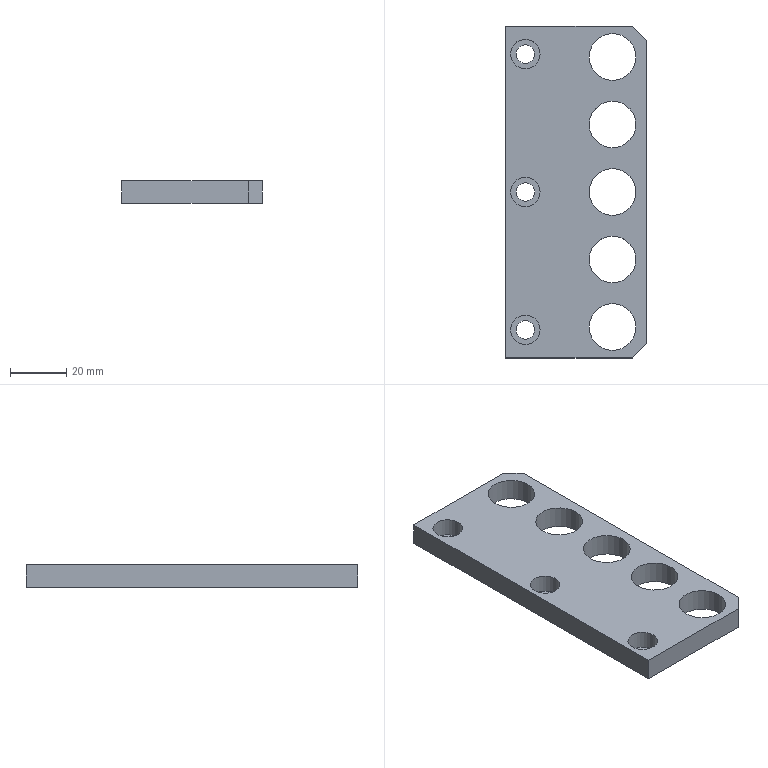NC program | NX | posted with a generic post | part box 50 x 118 x 8 mm
Lines 55 to 856 of 2555:
(ADAPTIVE_MILLING , TOOL : D8开粗)
N96 T04 M6
N98 G54
N100 G17 G0 G90 X50.236 Y10.179 S3500 M3
N102 G43 Z30. H4
N104 Z3.
N106 G94 G3 X50.236 Y10.179 Z2.605 I-2.237 J2.82 F1500.
N108 X50.236 Y10.179 Z2.21 I-2.237 J2.82
N110 X50.236 Y10.179 Z1.816 I-2.237 J2.82
N112 X50.236 Y10.179 Z1.421 I-2.237 J2.82
N114 X50.236 Y10.179 Z1.026 I-2.237 J2.82
N116 X50.236 Y10.179 Z0.631 I-2.237 J2.82
N118 X50.236 Y10.179 Z0.236 I-2.237 J2.82
N120 X50.236 Y10.179 Z-0.159 I-2.237 J2.82
N122 X50.236 Y10.179 Z-0.553 I-2.237 J2.82
N124 X50.236 Y10.179 Z-0.948 I-2.237 J2.82
N126 X50.236 Y10.179 Z-1.343 I-2.237 J2.82
N128 X50.236 Y10.179 Z-1.738 I-2.237 J2.82
N130 X50.236 Y10.179 Z-2.133 I-2.237 J2.82
N132 X50.236 Y10.179 Z-2.528 I-2.237 J2.82
N134 X50.236 Y10.179 Z-2.922 I-2.237 J2.82
N136 X50.236 Y10.179 Z-3.317 I-2.237 J2.82
N138 X50.236 Y10.179 Z-3.712 I-2.237 J2.82
N140 X50.236 Y10.179 Z-4.107 I-2.237 J2.82
N142 X50.236 Y10.179 Z-4.502 I-2.237 J2.82
N144 X50.236 Y10.179 Z-4.896 I-2.237 J2.82
N146 X50.236 Y10.179 Z-5.291 I-2.237 J2.82
N148 X50.236 Y10.179 Z-5.686 I-2.237 J2.82
N150 X50.236 Y10.179 Z-6.081 I-2.237 J2.82
N152 X50.236 Y10.179 Z-6.476 I-2.237 J2.82
N154 X50.236 Y10.179 Z-6.871 I-2.237 J2.82
N156 X50.236 Y10.179 Z-7.265 I-2.237 J2.82
N158 X50.236 Y10.179 Z-7.66 I-2.237 J2.82
N160 X50.236 Y10.179 Z-8.055 I-2.237 J2.82
N162 X50.236 Y10.179 Z-8.45 I-2.237 J2.82
N164 X50.236 Y10.179 Z-8.845 I-2.237 J2.82
N166 X47.998 Y16.599 Z-9. R3.6
N168 X51.279 Y11.397 R-3.625
N170 X44.716 Y11.182 R-3.701
N172 X49.182 Y16.615 R-3.777
N174 X45.263 Y10.239 R3.838
N176 X49.031 Y16.803 R-3.912
N178 X45.517 Y9.836 R3.976
N180 X49.277 Y16.867 R-4.046
N182 X45.642 Y9.575 R4.112
N184 X49.892 Y9.281 R4.161
N186 X44.448 Y15.226 R-4.182
N188 X44.68 Y10.442 R4.226
N190 X48.76 Y8.878 R4.238
N192 X51.89 Y11.457 R4.207
N194 X49.71 Y16.818 R4.18
N196 G1 X49.479 Y16.921
N198 G3 X48.429 Y16.246 R0.808
N200 G1 X48.303 Y15.168
N202 X48.286 Y15.019 Z-8.996
N204 X48.268 Y14.87 Z-8.985
N206 X48.251 Y14.721 Z-8.966
N208 X48.234 Y14.572 Z-8.939
N210 X48.216 Y14.423 Z-8.905
N212 X48.199 Y14.274 Z-8.862
N214 X48.181 Y14.125 Z-8.81
N216 X48.164 Y13.976 Z-8.75
N218 X48.147 Y13.827 Z-8.679
N220 X48.129 Y13.678 Z-8.598
N222 X48.112 Y13.529 Z-8.505
N224 X48.094 Y13.38 Z-8.4
N226 X48.077 Y13.231 Z-8.28
N228 X48.059 Y13.082 Z-8.142
N230 X48.042 Y12.933 Z-7.984
N232 X48.025 Y12.784 Z-7.8
N234 X48.007 Y12.635 Z-7.58
N236 X47.99 Y12.486 Z-7.308
N238 X47.972 Y12.337 Z-6.937
N240 X47.955 Y12.188 Z-6.
N242 G0 Z30.
N244 X26.236 Y10.182
N246 Z3.
N248 G3 X26.236 Y10.182 Z2.605 I-2.237 J2.82
N250 X26.236 Y10.182 Z2.21 I-2.237 J2.82
N252 X26.236 Y10.182 Z1.816 I-2.237 J2.82
N254 X26.236 Y10.182 Z1.421 I-2.237 J2.82
N256 X26.236 Y10.182 Z1.026 I-2.237 J2.82
N258 X26.236 Y10.182 Z0.631 I-2.237 J2.82
N260 X26.236 Y10.182 Z0.236 I-2.237 J2.82
N262 X26.236 Y10.182 Z-0.159 I-2.237 J2.82
N264 X26.236 Y10.182 Z-0.553 I-2.237 J2.82
N266 X26.236 Y10.182 Z-0.948 I-2.237 J2.82
N268 X26.236 Y10.182 Z-1.343 I-2.237 J2.82
N270 X26.236 Y10.182 Z-1.738 I-2.237 J2.82
N272 X26.236 Y10.182 Z-2.133 I-2.237 J2.82
N274 X26.236 Y10.182 Z-2.528 I-2.237 J2.82
N276 X26.236 Y10.182 Z-2.922 I-2.237 J2.82
N278 X26.236 Y10.182 Z-3.317 I-2.237 J2.82
N280 X26.236 Y10.182 Z-3.712 I-2.237 J2.82
N282 X26.236 Y10.182 Z-4.107 I-2.237 J2.82
N284 X26.236 Y10.182 Z-4.502 I-2.237 J2.82
N286 X26.236 Y10.182 Z-4.896 I-2.237 J2.82
N288 X26.236 Y10.182 Z-5.291 I-2.237 J2.82
N290 X26.236 Y10.182 Z-5.686 I-2.237 J2.82
N292 X26.236 Y10.182 Z-6.081 I-2.237 J2.82
N294 X26.236 Y10.182 Z-6.476 I-2.237 J2.82
N296 X26.236 Y10.182 Z-6.871 I-2.237 J2.82
N298 X26.236 Y10.182 Z-7.265 I-2.237 J2.82
N300 X26.236 Y10.182 Z-7.66 I-2.237 J2.82
N302 X26.236 Y10.182 Z-8.055 I-2.237 J2.82
N304 X26.236 Y10.182 Z-8.45 I-2.237 J2.82
N306 X26.236 Y10.182 Z-8.845 I-2.237 J2.82
N308 X23.999 Y16.602 Z-9. R3.6
N310 X27.28 Y11.4 R-3.625
N312 X20.716 Y11.186 R-3.701
N314 X25.184 Y16.62 R-3.778
N316 X21.42 Y10.095 R3.84
N318 X25.242 Y16.743 R-3.913
N320 X21.691 Y9.71 R3.978
N322 X25.282 Y16.871 R-4.048
N324 X21.826 Y9.459 R4.114
N326 X25.888 Y9.282 R4.161
N328 X21.511 Y16.374 R-4.181
N330 X27.568 Y15.195 R-4.189
N332 X26.569 Y16.317 R4.309
N334 X25.324 Y15.974 R0.808
N336 G1 X24.935 Y14.99
N338 X24.879 Y14.851 Z-8.996
N340 X24.824 Y14.711 Z-8.985
N342 X24.769 Y14.572 Z-8.966
N344 X24.714 Y14.432 Z-8.939
N346 X24.659 Y14.293 Z-8.905
N348 X24.604 Y14.153 Z-8.862
N350 X24.548 Y14.014 Z-8.81
N352 X24.493 Y13.874 Z-8.75
N354 X24.438 Y13.735 Z-8.679
N356 X24.383 Y13.595 Z-8.598
N358 X24.328 Y13.456 Z-8.505
N360 X24.273 Y13.316 Z-8.4
N362 X24.217 Y13.177 Z-8.28
N364 X24.162 Y13.037 Z-8.142
N366 X24.107 Y12.898 Z-7.984
N368 X24.052 Y12.758 Z-7.8
N370 X23.997 Y12.619 Z-7.58
N372 X23.942 Y12.479 Z-7.308
N374 X23.887 Y12.34 Z-6.937
N376 X23.831 Y12.2 Z-6.
N378 G0 Z30.
N380 X2.234 Y10.181
N382 Z3.
N384 G3 X2.234 Y10.181 Z2.605 I-2.237 J2.82
N386 X2.234 Y10.181 Z2.21 I-2.237 J2.82
N388 X2.234 Y10.181 Z1.816 I-2.237 J2.82
N390 X2.234 Y10.181 Z1.421 I-2.237 J2.82
N392 X2.234 Y10.181 Z1.026 I-2.237 J2.82
N394 X2.234 Y10.181 Z0.631 I-2.237 J2.82
N396 X2.234 Y10.181 Z0.236 I-2.237 J2.82
N398 X2.234 Y10.181 Z-0.159 I-2.237 J2.82
N400 X2.234 Y10.181 Z-0.553 I-2.237 J2.82
N402 X2.234 Y10.181 Z-0.948 I-2.237 J2.82
N404 X2.234 Y10.181 Z-1.343 I-2.237 J2.82
N406 X2.234 Y10.181 Z-1.738 I-2.237 J2.82
N408 X2.234 Y10.181 Z-2.133 I-2.237 J2.82
N410 X2.234 Y10.181 Z-2.528 I-2.237 J2.82
N412 X2.234 Y10.181 Z-2.922 I-2.237 J2.82
N414 X2.234 Y10.181 Z-3.317 I-2.237 J2.82
N416 X2.234 Y10.181 Z-3.712 I-2.237 J2.82
N418 X2.234 Y10.181 Z-4.107 I-2.237 J2.82
N420 X2.234 Y10.181 Z-4.502 I-2.237 J2.82
N422 X2.234 Y10.181 Z-4.896 I-2.237 J2.82
N424 X2.234 Y10.181 Z-5.291 I-2.237 J2.82
N426 X2.234 Y10.181 Z-5.686 I-2.237 J2.82
N428 X2.234 Y10.181 Z-6.081 I-2.237 J2.82
N430 X2.234 Y10.181 Z-6.476 I-2.237 J2.82
N432 X2.234 Y10.181 Z-6.871 I-2.237 J2.82
N434 X2.234 Y10.181 Z-7.265 I-2.237 J2.82
N436 X2.234 Y10.181 Z-7.66 I-2.237 J2.82
N438 X2.234 Y10.181 Z-8.055 I-2.237 J2.82
N440 X2.234 Y10.181 Z-8.45 I-2.237 J2.82
N442 X2.234 Y10.181 Z-8.845 I-2.237 J2.82
N444 X-0.003 Y16.601 Z-9. R3.6
N446 X3.277 Y11.399 R-3.625
N448 X-3.285 Y11.184 R-3.701
N450 X1.18 Y16.617 R-3.777
N452 X-2.739 Y10.241 R3.838
N454 X1.029 Y16.805 R-3.912
N456 X-2.125 Y9.586 R3.977
N458 X1.064 Y16.936 R-4.048
N460 X-2.172 Y9.455 R4.114
N462 X1.269 Y9.031 R4.161
N464 X-3.945 Y14.399 R-4.177
N466 X3.077 Y15.84 R-4.187
N468 X1.752 Y16.81 R4.235
N470 X0.622 Y16.2 R0.808
N472 G1 X0.455 Y15.146
N474 X0.432 Y14.998 Z-8.996
N476 X0.408 Y14.85 Z-8.985
N478 X0.385 Y14.702 Z-8.966
N480 X0.361 Y14.554 Z-8.939
N482 X0.338 Y14.406 Z-8.905
N484 X0.314 Y14.257 Z-8.862
N486 X0.291 Y14.109 Z-8.81
N488 X0.268 Y13.961 Z-8.75
N490 X0.244 Y13.813 Z-8.679
N492 X0.221 Y13.665 Z-8.598
N494 X0.197 Y13.517 Z-8.505
N496 X0.174 Y13.369 Z-8.4
N498 X0.15 Y13.22 Z-8.28
N500 X0.127 Y13.072 Z-8.142
N502 X0.104 Y12.924 Z-7.984
N504 X0.08 Y12.776 Z-7.8
N506 X0.057 Y12.628 Z-7.58
N508 X0.033 Y12.48 Z-7.308
N510 X0.01 Y12.331 Z-6.937
N512 X-0.013 Y12.183 Z-6.
N514 G0 Z30.
N516 X0.506 Y-39.041
N518 Z-6.
N520 G1 X0.507 Y-38.891 Z-6.937
N522 X0.509 Y-38.741 Z-7.308
N524 X0.51 Y-38.591 Z-7.58
N526 X0.512 Y-38.441 Z-7.8
N528 X0.513 Y-38.291 Z-7.984
N530 X0.514 Y-38.141 Z-8.142
N532 X0.516 Y-37.991 Z-8.28
N534 X0.517 Y-37.841 Z-8.4
N536 X0.519 Y-37.691 Z-8.505
N538 X0.52 Y-37.541 Z-8.598
N540 X0.522 Y-37.391 Z-8.679
N542 X0.523 Y-37.241 Z-8.75
N544 X0.525 Y-37.091 Z-8.81
N546 X0.526 Y-36.941 Z-8.862
N548 X0.528 Y-36.791 Z-8.905
N550 X0.529 Y-36.641 Z-8.939
N552 X0.53 Y-36.491 Z-8.966
N554 X0.532 Y-36.341 Z-8.985
N556 X0.533 Y-36.191 Z-8.996
N558 X0.535 Y-36.041 Z-9.
N560 X0.547 Y-34.792
N562 G3 X-0.008 Y-34.016 R0.808
N564 X-2.484 Y-33.75 R10.653
N566 X-8.994 Y-33.699 R394.13
N568 G1 X-61.118 Y-33.698
N570 G2 X-64.699 Y-31.591 R4.579
N572 X-65.979 Y-27.829 R8.408
N574 X-66.193 Y-22.211 R50.658
N576 G1 X-66.198 Y-18.011
N578 X-66.197 Y28.592
N580 G2 X-64.179 Y32.122 R4.565
N582 X-60.411 Y33.465 R8.23
N584 X-55.394 Y33.69 R42.849
N586 G1 X-50.444 Y33.699
N588 X61.106 Y33.698
N590 G2 X64.711 Y31.557 R4.596
N592 X65.982 Y27.78 R8.5
N594 X66.193 Y22.2 R50.827
N596 G1 X66.198 Y18.
N598 X66.197 Y-28.603
N600 G2 X64.092 Y-32.187 R4.584
N602 X60.338 Y-33.476 R8.406
N604 X54.72 Y-33.694 R49.804
N606 G1 X50.52 Y-33.699
N608 X1.745 Y-33.698
N610 G3 X-2.839 Y-33.457 R703.994
N612 X-10.268 Y-33.4 R435.247
N614 G1 X-59.656 Y-33.398
N616 G2 X-64.449 Y-30.442 R5.687
N618 X-65.692 Y-26.187 R10.577
N620 X-65.894 Y-20.043 R64.975
N622 G1 X-65.898 Y-16.743
N624 X-65.896 Y27.129
N626 G2 X-62.928 Y31.949 R5.7
N628 X-58.858 Y33.171 R10.376
N630 X-53.24 Y33.391 R54.557
N632 G1 X-49.115 Y33.399
N634 X59.64 Y33.397
N636 G2 X64.451 Y30.427 R5.7
N638 X65.674 Y26.324 R10.42
N640 X65.891 Y20.668 R55.859
N642 G1 X65.898 Y16.131
N644 X65.896 Y-27.14
N646 G2 X62.977 Y-31.922 R5.688
N648 X58.88 Y-33.169 R10.292
N650 X53.3 Y-33.391 R53.72
N652 G1 X49.175 Y-33.399
N654 X2.745 Y-33.396
N656 G2 X-3.054 Y-33.162 R769.478
N658 G3 X-11.206 Y-33.1 R473.739
N660 G1 X-58.381 Y-33.097
N662 G2 X-64.217 Y-29.458 R6.453
N664 X-65.394 Y-24.989 R12.24
N666 X-65.595 Y-18.094 R78.796
N668 G1 X-65.598 Y-14.382
N670 X-65.596 Y25.854
N672 G2 X-61.883 Y31.75 R6.483
N674 X-57.515 Y32.89 R12.302
N676 X-51.071 Y33.094 R72.384
N678 G1 X-47.771 Y33.098
N680 X58.365 Y33.097
N682 G2 X64.241 Y29.4 R6.471
N684 X65.387 Y25.036 R12.262
N686 X65.594 Y18.179 R76.142
N688 G1 X65.598 Y14.466
N690 X65.596 Y-25.865
N692 G2 X61.894 Y-31.747 R6.473
N694 X57.417 Y-32.9 R12.435
N696 X51.16 Y-33.094 R73.915
N698 G1 X47.86 Y-33.098
N700 X3.645 Y-33.096
N702 G2 X-3.124 Y-32.868 R440.519
N704 G3 X-11.918 Y-32.8 R494.43
N706 G1 X-57.168 Y-32.798
N708 G2 X-61.748 Y-31.398 R7.3
N710 X-64.538 Y-27.089 R8.183
N712 X-65.216 Y-22.123 R20.919
N714 X-65.298 Y-13.048 R277.677
N716 G1 X-65.296 Y24.692
N718 G2 X-63.836 Y29.32 R7.265
N720 X-59.558 Y32.045 R8.231
N722 X-54.516 Y32.72 R21.269
N724 X-45.929 Y32.798 R280.799
N726 G1 X57.146 Y32.797
N728 G2 X61.604 Y31.5 R7.358
N730 X64.495 Y27.22 R8.063
N732 X65.205 Y22.335 R19.927
N734 X65.298 Y13.373 R240.548
N736 G1 X65.296 Y-24.703
N738 G2 X63.784 Y-29.388 R7.242
N740 X59.421 Y-32.084 R8.332
N742 X54.56 Y-32.718 R21.674
N744 X45.823 Y-32.798 R276.552
N746 G1 X4.883
N748 G2 X-3.231 Y-32.571 R325.759
N750 G3 X-11.806 Y-32.5 R535.192
N752 G1 X-55.944 Y-32.499
N754 G2 X-59.694 Y-31.897 R9.494
N756 X-63.796 Y-27.611 R7.681
N758 X-64.814 Y-22.863 R15.69
N760 X-64.995 Y-15.329 R103.821
N762 G1 X-64.997 Y-12.029
N764 X-64.996 Y23.642
N766 G2 X-64.186 Y27.647 R8.751
N768 X-59.895 Y31.381 R7.847
N770 X-55.019 Y32.34 R16.701
N772 X-47.672 Y32.496 R117.542
N774 G1 X-44.785 Y32.498
N776 X56.152 Y32.496
N778 G2 X60.189 Y31.665 R8.695
N780 X63.885 Y27.383 R7.856
N782 X64.834 Y22.581 R16.635
N784 X64.995 Y15.197 R114.549
N786 G1 X64.997 Y11.897
N788 X64.996 Y-23.578
N790 G2 X64.279 Y-27.454 R8.997
N792 X59.975 Y-31.35 R7.776
N794 X55.178 Y-32.328 R16.273
N796 X47.119 Y-32.497 R119.876
N798 G1 X5.783 Y-32.498
N800 G2 X-3.449 Y-32.271 R353.509
N802 G3 X-12.818 Y-32.2 R603.998
N804 G1 X-55.106 Y-32.199
N806 G2 X-58.942 Y-31.636 R10.675
N808 X-63.378 Y-27.239 R7.929
N810 X-64.482 Y-22.397 R15.638
N812 X-64.694 Y-14.527 R97.762
N814 G1 X-64.697 Y-10.477
N816 X-64.696 Y22.554
N818 G2 X-64.15 Y26.394 R10.845
N820 X-59.743 Y30.874 R7.92
N822 X-54.715 Y31.999 R15.91
N824 X-47.482 Y32.194 R96.259
N826 G1 X-44.182 Y32.198
N828 X55.139 Y32.196
N830 G2 X58.974 Y31.62 R10.548
N832 X63.39 Y27.203 R7.945
N834 X64.501 Y22.17 R16.064
N836 X64.693 Y14.787 R100.086
N838 G1 X64.697 Y10.662
N840 X64.695 Y-22.64
N842 G2 X64.093 Y-26.544 R10.467
N844 X59.721 Y-30.884 R7.949
N846 X54.911 Y-31.981 R15.644
N848 X47.566 Y-32.194 R90.033
N850 G1 X44.266 Y-32.198
N852 X5.82 Y-32.196
N854 G2 X-4.038 Y-31.962 R549.5
N856 G3 X-12.968 Y-31.9 R639.08
N858 G1 X-54.056 Y-31.899
N860 G2 X-57.917 Y-31.47 R13.202
N862 X-62.997 Y-26.818 R8.147
N864 X-64.16 Y-21.875 R15.842
N866 X-64.389 Y-14.831 R83.45
N868 G1 X-64.397 Y-9.506
N870 X-64.395 Y21.719
N872 G2 X-63.906 Y25.609 R12.287
N874 X-59.313 Y30.497 R8.165
N876 X-54.295 Y31.668 R15.966
N878 X-46.764 Y31.893 R90.426
N880 G1 X-43.464 Y31.897
N882 X54.315 Y31.895
N884 G2 X58.234 Y31.364 R11.835
N886 X63.01 Y26.782 R8.183
N888 X64.163 Y21.837 R15.972
N890 X64.389 Y14.718 R84.962
N892 G1 X64.397 Y9.318
N894 X64.388 Y-22.653
N896 G2 X63.195 Y-27.17 R9.198
N898 X58.589 Y-30.789 R8.684
N900 X53.443 Y-31.737 R18.895
N902 X45.346 Y-31.896 R135.04
N904 G1 X7.433 Y-31.898
N906 G2 X-3.371 Y-31.679 R375.458
N908 G3 X-12.744 Y-31.601 R637.098
N910 G1 X-53.231 Y-31.599
N912 G2 X-57.175 Y-31.209 R14.957
N914 X-61.632 Y-28.13 R8.098
N916 G1 X-62.206 Y-27.556
N918 X-62.694 Y-26.779
N920 G2 X-63.913 Y-20.641 R21.436
N922 X-64.092 Y-12.844 R123.731
N924 G1 X-64.097 Y-8.794
N926 X-64.095 Y20.867
N928 G2 X-63.658 Y24.841 R14.049
N930 X-58.868 Y30.14 R8.396
N932 X-53.819 Y31.346 R16.185
N934 X-45.988 Y31.592 R88.752
N936 G1 X-41.863 Y31.597
N938 X53.452 Y31.595
N940 G2 X57.423 Y31.134 R13.608
N942 X62.656 Y26.33 R8.411
N944 X63.848 Y21.278 R16.311
N946 X64.088 Y13.934 R85.558
N948 G1 X64.096 Y8.61
N950 X64.095 Y-22.453
N952 G2 X62.534 Y-27.202 R9.265
N954 X57.722 Y-30.583 R9.267
N956 X52.483 Y-31.451 R21.049
N958 X42.585 Y-31.597 R188.242
N960 G1 X6.898 Y-31.596
N962 G2 X-3.999 Y-31.369 R550.68
N964 G3 X-13.269 Y-31.301 R647.104
N966 G1 X-52.331 Y-31.3
N968 G2 X-56.285 Y-30.984 R17.939
N970 X-60.293 Y-28.883 R9.158
N972 X-61.556 Y-28.206 R4.98
N974 G1 X-62.206 Y-27.556
N976 X-62.694 Y-26.779
N978 X-62.997 Y-25.912
N980 G2 X-63.575 Y-20.794 R161.787
N982 X-63.792 Y-11.724 R131.889
N984 G1 X-63.796 Y-7.449
N986 X-63.795 Y19.967
N988 G2 X-63.421 Y24.026 R16.509
N990 X-58.473 Y29.772 R8.603
N992 X-53.395 Y31.021 R16.295
N994 X-46.091 Y31.288 R78.704
N996 G1 X-41.028 Y31.297
N998 X52.627 Y31.295
N1000 G2 X56.717 Y30.871 R15.336
N1002 X62.268 Y25.981 R8.606
N1004 X63.529 Y20.793 R16.411
N1006 X63.787 Y13.15 R85.647
N1008 G1 X63.796 Y8.2
N1010 X63.795 Y-22.45
N1012 G2 X63.072 Y-25.258 R13.964
N1014 G1 X63.002 Y-25.889
N1016 G2 X62.249 Y-27.501 R4.767
N1018 X60.884 Y-28.641 R4.767
N1020 X54.012 Y-30.958 R16.079
N1022 X47.011 Y-31.282 R64.531
N1024 G1 X40.973 Y-31.297
N1026 X7.461 Y-31.296
N1028 G2 X-4.48 Y-31.063 R634.025
N1030 G3 X-13.793 Y-31.001 R655.45
N1032 G1 X-51.506 Y-31.
N1034 G2 X-55.686 Y-30.689 R19.936
N1036 X-59.197 Y-29.18 R11.272
N1038 G3 X-59.912 Y-28.997 R1.401
N1040 G1 X-60.779 Y-28.694
N1042 X-61.556 Y-28.206
N1044 X-62.206 Y-27.556
N1046 X-62.694 Y-26.779
N1048 X-62.997 Y-25.912
N1050 G2 X-63.102 Y-23.654 R12.983
N1052 X-63.449 Y-16.244 R192.047
N1054 X-63.496 Y-6.644 R677.077
N1056 G1 X-63.495 Y19.131
N1058 G2 X-63.165 Y23.271 R18.98
N1060 X-58.014 Y29.443 R8.819
N1062 X-52.753 Y30.721 R16.806
N1064 X-45.148 Y30.989 R83.609
N1066 G1 X-40.198 Y30.997
N1068 X51.727 Y30.996
N1070 G2 X55.902 Y30.636 R18.017
N1072 X61.933 Y25.534 R8.815
N1074 X63.224 Y20.2 R16.866
N1076 X63.487 Y12.219 R90.237
N1078 G1 X63.496 Y6.819
N1080 X63.494 Y-22.443
N1082 X63.1 Y-24.093
N1084 G2 X63.071 Y-25.262 R9.795
N1086 G3 X63.58 Y-26.103 R0.808
N1088 G1 X64.859 Y-26.602
N1090 X64.998 Y-26.656 Z-8.996
N1092 X65.138 Y-26.711 Z-8.985
N1094 X65.278 Y-26.766 Z-8.966
N1096 X65.417 Y-26.82 Z-8.939
N1098 X65.557 Y-26.875 Z-8.905
N1100 X65.697 Y-26.929 Z-8.862
N1102 X65.837 Y-26.984 Z-8.81
N1104 X65.976 Y-27.038 Z-8.75
N1106 X66.116 Y-27.093 Z-8.679
N1108 X66.256 Y-27.148 Z-8.598
N1110 X66.395 Y-27.202 Z-8.505
N1112 X66.535 Y-27.257 Z-8.4
N1114 X66.675 Y-27.311 Z-8.28
N1116 X66.815 Y-27.366 Z-8.142
N1118 X66.954 Y-27.421 Z-7.984
N1120 X67.094 Y-27.475 Z-7.8
N1122 X67.234 Y-27.53 Z-7.58
N1124 X67.373 Y-27.584 Z-7.308
N1126 X67.513 Y-27.639 Z-6.937
N1128 X67.653 Y-27.693 Z-6.
N1130 G0 Z30.
N1132 X-67.881 Y-23.617
N1134 Z-6.
N1136 G1 X-67.741 Y-23.671 Z-6.937
N1138 X-67.602 Y-23.726 Z-7.308
N1140 X-67.462 Y-23.78 Z-7.58
N1142 X-67.322 Y-23.835 Z-7.8
N1144 X-67.183 Y-23.89 Z-7.984
N1146 X-67.043 Y-23.944 Z-8.142
N1148 X-66.903 Y-23.999 Z-8.28
N1150 X-66.763 Y-24.053 Z-8.4
N1152 X-66.624 Y-24.108 Z-8.505
N1154 X-66.484 Y-24.162 Z-8.598
N1156 X-66.344 Y-24.217 Z-8.679
N1158 X-66.204 Y-24.272 Z-8.75
N1160 X-66.065 Y-24.326 Z-8.81
N1162 X-65.925 Y-24.381 Z-8.862
N1164 X-65.785 Y-24.435 Z-8.905
N1166 X-65.646 Y-24.49 Z-8.939
N1168 X-65.506 Y-24.544 Z-8.966
N1170 X-65.366 Y-24.599 Z-8.985
N1172 X-65.226 Y-24.654 Z-8.996
N1174 X-65.087 Y-24.708 Z-9.
N1176 G3 X-64.62 Y-24.745 R0.821
N1178 G1 X-63.735 Y-24.551
N1180 G3 X-63.1 Y-23.762 R0.808
N1182 X-63.186 Y-12.277 R757.047
N1184 G1 X-63.196 Y-7.027
N1186 X-63.194 Y18.46
N1188 G2 X-62.858 Y22.751 R20.089
N1190 X-57.536 Y29.129 R9.028
N1192 X-52.087 Y30.427 R17.438
N1194 X-44.144 Y30.689 R90.646
N1196 G1 X-38.819 Y30.697
N1198 X50.977 Y30.695
N1200 G2 X55.194 Y30.371 R20.248
N1202 X61.633 Y25.025 R9.029
N1204 X62.605 Y21.917 R16.705
N1206 X63.021 Y20.798 R4.271
N1208 X63.1 Y18.349 R16.852
N1210 X63.196 Y5.708 R594.316
N1212 G1 X63.194 Y-21.755
N1214 X63.1 Y-22.369
N1216 Y-24.094
N1218 G3 X64.658 Y-24.35 R0.8
N1220 G1 X65.083 Y-22.818 Z-8.9
N1222 X65.201 Y-22.406 F15000.
N1224 X65.305 Y-21.989
N1226 X65.313 Y-21.882
N1228 Y16.137
N1230 X65.303 Y16.244
N1232 X65.284 Y16.35
N1234 X65.09 Y17.048
N1236 X64.666 Y18.58 Z-9. F1500.
N1238 G3 X63.1 Y18.349 R0.8
N1240 G1 Y-25.001
N1242 G2 X62.714 Y-26.736 R4.764
N1244 X61.629 Y-28.146 R4.767
N1246 X60.048 Y-28.964 R4.764
N1248 X51.534 Y-30.833 R25.207
N1250 X42.274 Y-30.996 R166.344
N1252 G1 X8.837 Y-30.997
N1254 G2 X-3.923 Y-30.775 R514.516
N1256 G3 X-14.656 Y-30.701 R680.231
N1258 G1 X-50.756 Y-30.7
N1260 G2 X-55.014 Y-30.412 R22.291
N1262 X-58.352 Y-29.226 R15.336
N1264 G3 X-59.001 Y-29.1 R1.258
N1266 X-59.753 Y-29.038 R13.408
N1268 G1 X-60.795 Y-29.171
N1270 G3 X-60.96 Y-30.736 R0.808
N1272 G1 X-60.818 Y-30.785 Z-8.996
N1274 X-60.677 Y-30.835 Z-8.985
N1276 X-60.535 Y-30.884 Z-8.966
N1278 X-60.393 Y-30.934 Z-8.939
N1280 X-60.252 Y-30.983 Z-8.905
N1282 X-60.11 Y-31.033 Z-8.862
N1284 X-59.969 Y-31.082 Z-8.81
N1286 X-59.827 Y-31.132 Z-8.75
N1288 X-59.686 Y-31.181 Z-8.679
N1290 X-59.544 Y-31.231 Z-8.598
N1292 X-59.402 Y-31.281 Z-8.505
N1294 X-59.261 Y-31.33 Z-8.4
N1296 X-59.119 Y-31.38 Z-8.28
N1298 X-58.978 Y-31.429 Z-8.142
N1300 X-58.836 Y-31.479 Z-7.984
N1302 X-58.694 Y-31.528 Z-7.8
N1304 X-58.553 Y-31.578 Z-7.58
N1306 X-58.411 Y-31.627 Z-7.308
N1308 X-58.27 Y-31.677 Z-6.937
N1310 X-58.128 Y-31.726 Z-6.
N1312 G0 Z30.
N1314 X58.764 Y-31.588
N1316 Z-6.
N1318 G1 X58.904 Y-31.534 Z-6.937
N1320 X59.044 Y-31.48 Z-7.308
N1322 X59.184 Y-31.426 Z-7.58
N1324 X59.324 Y-31.372 Z-7.8
N1326 X59.464 Y-31.318 Z-7.984
N1328 X59.604 Y-31.264 Z-8.142
N1330 X59.743 Y-31.21 Z-8.28
N1332 X59.883 Y-31.156 Z-8.4
N1334 X60.023 Y-31.102 Z-8.505
N1336 X60.163 Y-31.048 Z-8.598
N1338 X60.303 Y-30.995 Z-8.679
N1340 X60.443 Y-30.941 Z-8.75
N1342 X60.583 Y-30.887 Z-8.81
N1344 X60.723 Y-30.833 Z-8.862
N1346 X60.863 Y-30.779 Z-8.905
N1348 X61.003 Y-30.725 Z-8.939
N1350 X61.143 Y-30.671 Z-8.966
N1352 X61.283 Y-30.617 Z-8.985
N1354 X61.423 Y-30.563 Z-8.996
N1356 X61.563 Y-30.509 Z-9.
N1358 G3 X61.271 Y-28.947 R0.808
N1360 G1 X60.048 Y-28.964
N1362 G3 X56.651 Y-29.77 R69.655
N1364 G2 X48.987 Y-30.623 R38.617
N1366 X39.687 Y-30.696 R423.148
N1368 G1 X8.2 Y-30.695
N1370 G2 X-4.369 Y-30.47 R687.903
N1372 G3 X-16.006 Y-30.401 R715.492
N1374 G1 X-56.406
N1376 X-56.694 Y-30.348
N1378 X-58.89 Y-29.511
N1380 G3 X-59.269 Y-31.069 R-0.808
N1382 G1 X-59.12 Y-31.086 Z-8.996
N1384 X-58.97 Y-31.103 Z-8.985
N1386 X-58.821 Y-31.119 Z-8.966
N1388 X-58.672 Y-31.136 Z-8.939
N1390 X-58.523 Y-31.153 Z-8.905
N1392 X-58.374 Y-31.17 Z-8.862
N1394 X-58.225 Y-31.187 Z-8.81
N1396 X-58.076 Y-31.203 Z-8.75
N1398 X-57.927 Y-31.22 Z-8.679
N1400 X-57.778 Y-31.237 Z-8.598
N1402 X-57.629 Y-31.254 Z-8.505
N1404 X-57.48 Y-31.271 Z-8.4
N1406 X-57.331 Y-31.287 Z-8.28
N1408 X-57.182 Y-31.304 Z-8.142
N1410 X-57.033 Y-31.321 Z-7.984
N1412 X-56.884 Y-31.338 Z-7.8
N1414 X-56.735 Y-31.355 Z-7.58
N1416 X-56.586 Y-31.371 Z-7.308
N1418 X-56.437 Y-31.388 Z-6.937
N1420 X-56.287 Y-31.405 Z-6.
N1422 G0 Z30.
N1424 X58.119 Y-31.837
N1426 Z-6.
N1428 G1 X58.259 Y-31.783 Z-6.937
N1430 X58.399 Y-31.729 Z-7.308
N1432 X58.539 Y-31.675 Z-7.58
N1434 X58.678 Y-31.621 Z-7.8
N1436 X58.818 Y-31.567 Z-7.984
N1438 X58.958 Y-31.513 Z-8.142
N1440 X59.098 Y-31.459 Z-8.28
N1442 X59.238 Y-31.405 Z-8.4
N1444 X59.378 Y-31.351 Z-8.505
N1446 X59.518 Y-31.297 Z-8.598
N1448 X59.658 Y-31.243 Z-8.679
N1450 X59.798 Y-31.189 Z-8.75
N1452 X59.938 Y-31.135 Z-8.81
N1454 X60.078 Y-31.081 Z-8.862
N1456 X60.218 Y-31.027 Z-8.905
N1458 X60.358 Y-30.973 Z-8.939
N1460 X60.498 Y-30.919 Z-8.966
N1462 X60.638 Y-30.866 Z-8.985
N1464 X60.778 Y-30.812 Z-8.996
N1466 X60.918 Y-30.758 Z-9.
N1468 G3 X60.728 Y-29.202 R0.808
N1470 G1 X59.528 Y-29.066
N1472 G3 X56.363 Y-29.539 R21.375
N1474 G2 X47.336 Y-30.349 R51.747
N1476 X38.261 Y-30.396 R658.085
N1478 G1 X-54.484 Y-30.394
N1480 G2 X-56.42 Y-29.693 R14.547
N1482 G3 X-58. Y-29.104 R11.805
N1484 X-58.986 Y-29.123 R9.512
N1486 G1 X-60.107 Y-29.399
N1488 G3 X-60.004 Y-30.986 R0.808
N1490 G1 X-59.855 Y-31.003 Z-8.996
N1492 X-59.706 Y-31.02 Z-8.985
N1494 X-59.557 Y-31.037 Z-8.966
N1496 X-59.408 Y-31.053 Z-8.939
N1498 X-59.259 Y-31.07 Z-8.905
N1500 X-59.11 Y-31.087 Z-8.862
N1502 X-58.961 Y-31.104 Z-8.81
N1504 X-58.812 Y-31.121 Z-8.75
N1506 X-58.663 Y-31.137 Z-8.679
N1508 X-58.514 Y-31.154 Z-8.598
N1510 X-58.365 Y-31.171 Z-8.505
N1512 X-58.216 Y-31.188 Z-8.4
N1514 X-58.067 Y-31.204 Z-8.28
N1516 X-57.917 Y-31.221 Z-8.142
N1518 X-57.768 Y-31.238 Z-7.984
N1520 X-57.619 Y-31.255 Z-7.8
N1522 X-57.47 Y-31.272 Z-7.58
N1524 X-57.321 Y-31.288 Z-7.308
N1526 X-57.172 Y-31.305 Z-6.937
N1528 X-57.023 Y-31.322 Z-6.
N1530 G0 Z30.
N1532 X57.318 Y-31.525
N1534 Z-6.
N1536 G1 X57.465 Y-31.496 Z-6.937
N1538 X57.612 Y-31.467 Z-7.308
N1540 X57.759 Y-31.438 Z-7.58
N1542 X57.906 Y-31.409 Z-7.8
N1544 X58.054 Y-31.38 Z-7.984
N1546 X58.201 Y-31.351 Z-8.142
N1548 X58.348 Y-31.322 Z-8.28
N1550 X58.495 Y-31.293 Z-8.4
N1552 X58.642 Y-31.264 Z-8.505
N1554 X58.79 Y-31.235 Z-8.598
N1556 X58.937 Y-31.207 Z-8.679
N1558 X59.084 Y-31.178 Z-8.75
N1560 X59.231 Y-31.149 Z-8.81
N1562 X59.378 Y-31.12 Z-8.862
N1564 X59.525 Y-31.091 Z-8.905
N1566 X59.673 Y-31.062 Z-8.939
N1568 X59.82 Y-31.033 Z-8.966
N1570 X59.967 Y-31.004 Z-8.985
N1572 X60.114 Y-30.975 Z-8.996
N1574 X60.261 Y-30.946 Z-9.
N1576 G3 X60.281 Y-29.365 R0.808
N1578 G1 X59. Y-29.1
N1580 G3 X55.818 Y-29.363 R17.161
N1582 G2 X45.539 Y-30.068 R71.47
N1584 G1 X37.214 Y-30.096
N1586 X-55.78 Y-30.106
N1588 X-56.032 Y-30.184
N1590 G3 X-56.329 Y-31.534 Z-8.9 R0.882
N1592 X-55.64 Y-31.856 R0.882 F15000.
N1594 G1 X32.259 Y-31.087
N1596 X33.848 Y-31.073 Z-9. F1500.
N1598 X58.182 Y-30.86
N1600 G3 X59.054 Y-29.972 R0.88
N1602 X58.175 Y-29.1 R0.88
N1604 X53.654 Y-29.352 R31.704
N1606 G2 X42.942 Y-29.784 R110.783
N1608 G1 X36.417 Y-29.796
N1610 X-55.79 Y-29.806
N1612 X-56.042 Y-29.884
N1614 G3 X-56.339 Y-31.234 Z-8.9 R0.882
N1616 X-55.653 Y-31.556 R0.882 F15000.
N1618 G1 X20.069 Y-31.087
N1620 X21.659 Y-31.077 Z-9. F1500.
N1622 X56.68 Y-30.86
N1624 G3 X57.555 Y-29.975 R0.88
N1626 X56.675 Y-29.1 R0.88
N1628 X50.737 Y-29.283 R64.589
N1630 G2 X39.716 Y-29.493 R214.643
N1632 G1 X35.741 Y-29.496
N1634 X-55.697 Y-29.494
N1636 X-57.053 Y-29.104
N1638 X-58.066 Y-29.1
N1640 G3 X-58.862 Y-29.984 R0.8
N1642 X-58.468 Y-30.596 Z-8.953 R0.839
N1644 G1 X-57.787 Y-31.08 Z-8.9
N1646 X-56.969 Y-31.662 F15000.
N1648 G3 X-56.502 Y-31.81 R0.81
N1650 G1 X52.062 Y-31.313
N1652 X52.271 Y-31.284
N1654 X52.971 Y-31.09
N1656 X54.503 Y-30.667 Z-9. F1500.
N1658 G3 X54.275 Y-29.1 R0.8
N1660 X41.661 Y-29.185 R835.77
N1662 G1 X35.136 Y-29.195
N1664 X-54.727 Y-29.193
N1666 X-55.357 Y-29.1
N1668 X-57.12
N1670 G3 X-57.375 Y-30.658 R0.8
N1672 G1 X-55.843 Y-31.083 Z-8.9
N1674 X-55.431 Y-31.201 F15000.
N1676 X-55.015 Y-31.305
N1678 X-54.907 Y-31.313
N1680 X46.399
N1682 X46.507 Y-31.303
N1684 X46.613 Y-31.284
N1686 X47.311 Y-31.09
N1688 X48.843 Y-30.666 Z-9. F1500.
N1690 G3 X48.612 Y-29.1 R0.8
N1692 G1 X-55.375